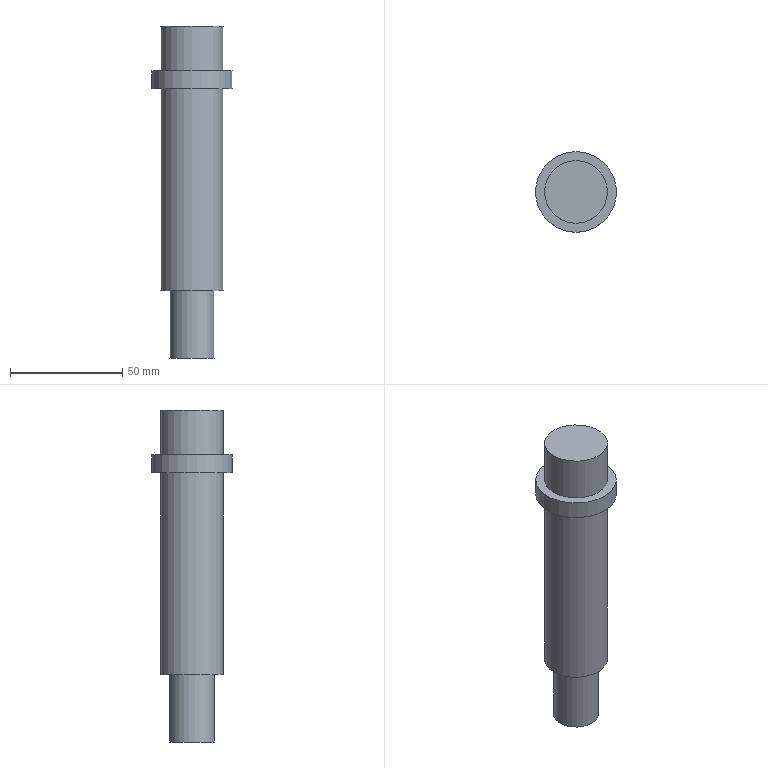Part | NX | features solid 2 | 1 solid | 9 faces | box 36 x 36 x 148 mm | volume 85301 mm3 | plane 5 | cylinder 4 | commonest cylinder face diameters 28 x2 20 x1 36 x1
STEP:
#1=CARTESIAN_POINT('',(200.,264.,308.));
#2=VERTEX_POINT('',#1);
#3=CARTESIAN_POINT('',(200.,250.,308.));
#4=DIRECTION('',(0.,0.,-1.));
#5=DIRECTION('',(0.,1.,0.));
#6=AXIS2_PLACEMENT_3D('',#3,#4,#5);
#7=CIRCLE('',#6,14.);
#8=EDGE_CURVE('',#2,#2,#7,.T.);
#9=ORIENTED_EDGE('',*,*,#8,.F.);
#10=EDGE_LOOP('',(#9));
#11=FACE_BOUND('',#10,.T.);
#12=CARTESIAN_POINT('',(200.,250.,308.));
#13=DIRECTION('',(0.,0.,1.));
#14=DIRECTION('',(0.,-1.,0.));
#15=AXIS2_PLACEMENT_3D('',#12,#13,#14);
#16=PLANE('',#15);
#17=ADVANCED_FACE('',(#11),#16,.T.);
#18=ORIENTED_EDGE('',*,*,#8,.T.);
#19=EDGE_LOOP('',(#18));
#20=FACE_BOUND('',#19,.T.);
#21=CARTESIAN_POINT('',(200.,236.,288.));
#22=VERTEX_POINT('',#21);
#23=CARTESIAN_POINT('',(200.,250.,288.));
#24=DIRECTION('',(0.,0.,1.));
#25=DIRECTION('',(0.,-1.,0.));
#26=AXIS2_PLACEMENT_3D('',#23,#24,#25);
#27=CIRCLE('',#26,14.);
#28=EDGE_CURVE('',#22,#22,#27,.F.);
#29=ORIENTED_EDGE('',*,*,#28,.F.);
#30=EDGE_LOOP('',(#29));
#31=FACE_BOUND('',#30,.T.);
#32=CARTESIAN_POINT('',(200.,250.,288.));
#33=DIRECTION('',(0.,0.,1.));
#34=DIRECTION('',(0.,-1.,0.));
#35=AXIS2_PLACEMENT_3D('',#32,#33,#34);
#36=CYLINDRICAL_SURFACE('',#35,14.);
#37=ADVANCED_FACE('',(#20,#31),#36,.T.);
#38=ORIENTED_EDGE('',*,*,#28,.T.);
#39=EDGE_LOOP('',(#38));
#40=FACE_BOUND('',#39,.T.);
#41=CARTESIAN_POINT('',(200.,268.,288.));
#42=VERTEX_POINT('',#41);
#43=CARTESIAN_POINT('',(200.,250.,288.));
#44=DIRECTION('',(0.,0.,-1.));
#45=DIRECTION('',(0.,1.,0.));
#46=AXIS2_PLACEMENT_3D('',#43,#44,#45);
#47=CIRCLE('',#46,18.);
#48=EDGE_CURVE('',#42,#42,#47,.T.);
#49=ORIENTED_EDGE('',*,*,#48,.F.);
#50=EDGE_LOOP('',(#49));
#51=FACE_BOUND('',#50,.T.);
#52=CARTESIAN_POINT('',(200.,250.,288.));
#53=DIRECTION('',(0.,0.,1.));
#54=DIRECTION('',(0.,-1.,0.));
#55=AXIS2_PLACEMENT_3D('',#52,#53,#54);
#56=PLANE('',#55);
#57=ADVANCED_FACE('',(#40,#51),#56,.T.);
#58=CARTESIAN_POINT('',(200.,264.,280.));
#59=VERTEX_POINT('',#58);
#60=CARTESIAN_POINT('',(200.,250.,280.));
#61=DIRECTION('',(0.,0.,-1.));
#62=DIRECTION('',(0.,1.,0.));
#63=AXIS2_PLACEMENT_3D('',#60,#61,#62);
#64=CIRCLE('',#63,14.);
#65=EDGE_CURVE('',#59,#59,#64,.T.);
#66=ORIENTED_EDGE('',*,*,#65,.F.);
#67=EDGE_LOOP('',(#66));
#68=FACE_BOUND('',#67,.T.);
#69=CARTESIAN_POINT('',(200.,232.,280.));
#70=VERTEX_POINT('',#69);
#71=CARTESIAN_POINT('',(200.,250.,280.));
#72=DIRECTION('',(0.,0.,1.));
#73=DIRECTION('',(0.,-1.,0.));
#74=AXIS2_PLACEMENT_3D('',#71,#72,#73);
#75=CIRCLE('',#74,18.);
#76=EDGE_CURVE('',#70,#70,#75,.T.);
#77=ORIENTED_EDGE('',*,*,#76,.F.);
#78=EDGE_LOOP('',(#77));
#79=FACE_BOUND('',#78,.T.);
#80=CARTESIAN_POINT('',(200.,250.,280.));
#81=DIRECTION('',(0.,0.,-1.));
#82=DIRECTION('',(0.,1.,0.));
#83=AXIS2_PLACEMENT_3D('',#80,#81,#82);
#84=PLANE('',#83);
#85=ADVANCED_FACE('',(#68,#79),#84,.T.);
#86=ORIENTED_EDGE('',*,*,#48,.T.);
#87=EDGE_LOOP('',(#86));
#88=FACE_BOUND('',#87,.T.);
#89=ORIENTED_EDGE('',*,*,#76,.T.);
#90=EDGE_LOOP('',(#89));
#91=FACE_BOUND('',#90,.T.);
#92=CARTESIAN_POINT('',(200.,250.,280.));
#93=DIRECTION('',(0.,0.,1.));
#94=DIRECTION('',(0.,-1.,0.));
#95=AXIS2_PLACEMENT_3D('',#92,#93,#94);
#96=CYLINDRICAL_SURFACE('',#95,18.);
#97=ADVANCED_FACE('',(#88,#91),#96,.T.);
#98=CARTESIAN_POINT('',(200.,260.,190.));
#99=VERTEX_POINT('',#98);
#100=CARTESIAN_POINT('',(200.,250.,190.));
#101=DIRECTION('',(0.,0.,-1.));
#102=DIRECTION('',(0.,1.,0.));
#103=AXIS2_PLACEMENT_3D('',#100,#101,#102);
#104=CIRCLE('',#103,10.);
#105=EDGE_CURVE('',#99,#99,#104,.T.);
#106=ORIENTED_EDGE('',*,*,#105,.F.);
#107=EDGE_LOOP('',(#106));
#108=FACE_BOUND('',#107,.T.);
#109=CARTESIAN_POINT('',(200.,236.,190.));
#110=VERTEX_POINT('',#109);
#111=CARTESIAN_POINT('',(200.,250.,190.));
#112=DIRECTION('',(0.,0.,1.));
#113=DIRECTION('',(0.,-1.,0.));
#114=AXIS2_PLACEMENT_3D('',#111,#112,#113);
#115=CIRCLE('',#114,14.);
#116=EDGE_CURVE('',#110,#110,#115,.T.);
#117=ORIENTED_EDGE('',*,*,#116,.F.);
#118=EDGE_LOOP('',(#117));
#119=FACE_BOUND('',#118,.T.);
#120=CARTESIAN_POINT('',(200.,250.,190.));
#121=DIRECTION('',(0.,0.,-1.));
#122=DIRECTION('',(0.,1.,0.));
#123=AXIS2_PLACEMENT_3D('',#120,#121,#122);
#124=PLANE('',#123);
#125=ADVANCED_FACE('',(#108,#119),#124,.T.);
#126=ORIENTED_EDGE('',*,*,#65,.T.);
#127=EDGE_LOOP('',(#126));
#128=FACE_BOUND('',#127,.T.);
#129=ORIENTED_EDGE('',*,*,#116,.T.);
#130=EDGE_LOOP('',(#129));
#131=FACE_BOUND('',#130,.T.);
#132=CARTESIAN_POINT('',(200.,250.,190.));
#133=DIRECTION('',(0.,0.,1.));
#134=DIRECTION('',(0.,-1.,0.));
#135=AXIS2_PLACEMENT_3D('',#132,#133,#134);
#136=CYLINDRICAL_SURFACE('',#135,14.);
#137=ADVANCED_FACE('',(#128,#131),#136,.T.);
#138=CARTESIAN_POINT('',(200.,240.,160.));
#139=VERTEX_POINT('',#138);
#140=CARTESIAN_POINT('',(200.,250.,160.));
#141=DIRECTION('',(0.,0.,1.));
#142=DIRECTION('',(0.,-1.,0.));
#143=AXIS2_PLACEMENT_3D('',#140,#141,#142);
#144=CIRCLE('',#143,10.);
#145=EDGE_CURVE('',#139,#139,#144,.T.);
#146=ORIENTED_EDGE('',*,*,#145,.F.);
#147=EDGE_LOOP('',(#146));
#148=FACE_BOUND('',#147,.T.);
#149=CARTESIAN_POINT('',(200.,250.,160.));
#150=DIRECTION('',(0.,0.,-1.));
#151=DIRECTION('',(0.,1.,0.));
#152=AXIS2_PLACEMENT_3D('',#149,#150,#151);
#153=PLANE('',#152);
#154=ADVANCED_FACE('',(#148),#153,.T.);
#155=ORIENTED_EDGE('',*,*,#105,.T.);
#156=EDGE_LOOP('',(#155));
#157=FACE_BOUND('',#156,.T.);
#158=ORIENTED_EDGE('',*,*,#145,.T.);
#159=EDGE_LOOP('',(#158));
#160=FACE_BOUND('',#159,.T.);
#161=CARTESIAN_POINT('',(200.,250.,160.));
#162=DIRECTION('',(0.,0.,1.));
#163=DIRECTION('',(0.,-1.,0.));
#164=AXIS2_PLACEMENT_3D('',#161,#162,#163);
#165=CYLINDRICAL_SURFACE('',#164,10.);
#166=ADVANCED_FACE('',(#157,#160),#165,.T.);
#167=CLOSED_SHELL('',(#17,#37,#57,#85,#97,#125,#137,#154,#166));
#168=MANIFOLD_SOLID_BREP('',#167);
#169=(LENGTH_UNIT()NAMED_UNIT(*)SI_UNIT(.MILLI.,.METRE.));
#170=UNCERTAINTY_MEASURE_WITH_UNIT(LENGTH_MEASURE(0.00001),#169,'','');
#171=(NAMED_UNIT(*)PLANE_ANGLE_UNIT()SI_UNIT($,.RADIAN.));
#172=(NAMED_UNIT(*)SI_UNIT($,.STERADIAN.)SOLID_ANGLE_UNIT());
#173=(GEOMETRIC_REPRESENTATION_CONTEXT(3)GLOBAL_UNCERTAINTY_ASSIGNED_CONTEXT((#170))GLOBAL_UNIT_ASSIGNED_CONTEXT((#169,#171,#172))REPRESENTATION_CONTEXT('',''));
#174=ADVANCED_BREP_SHAPE_REPRESENTATION('',(#168),#173);